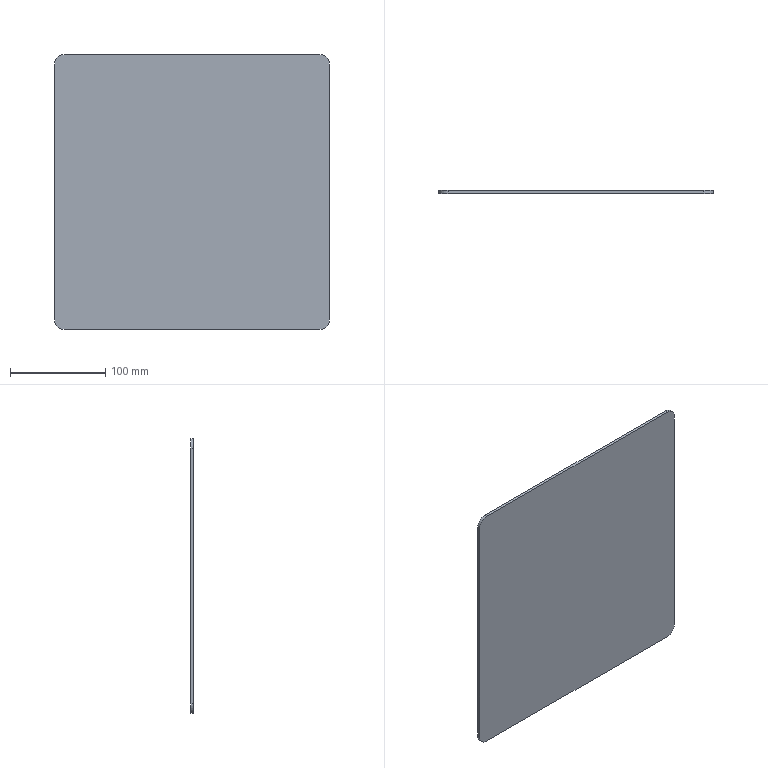Part | SolidWorks | features Extrusion 1 | 1 solid | 10 faces | box 288 x 3 x 288 mm | volume 248574 mm3 | plane 6 | cylinder 4 | commonest cylinder face diameters 20 x4
STEP:
#1=CARTESIAN_POINT('',(-144.,0.,134.));
#2=VERTEX_POINT('',#1);
#3=CARTESIAN_POINT('',(-134.,0.,144.));
#4=VERTEX_POINT('',#3);
#5=CARTESIAN_POINT('',(-134.,0.,134.));
#6=DIRECTION('',(0.,1.,0.));
#7=DIRECTION('',(0.,0.,-1.));
#8=AXIS2_PLACEMENT_3D('',#5,#6,#7);
#9=CIRCLE('',#8,10.);
#10=EDGE_CURVE('',#2,#4,#9,.T.);
#11=ORIENTED_EDGE('',*,*,#10,.T.);
#12=CARTESIAN_POINT('',(-134.,3.,144.));
#13=VERTEX_POINT('',#12);
#14=CARTESIAN_POINT('',(-134.,3.,144.));
#15=DIRECTION('',(0.,-1.,0.));
#16=VECTOR('',#15,1000.);
#17=LINE('',#14,#16);
#18=EDGE_CURVE('',#13,#4,#17,.T.);
#19=ORIENTED_EDGE('',*,*,#18,.F.);
#20=CARTESIAN_POINT('',(-144.,3.,134.));
#21=VERTEX_POINT('',#20);
#22=CARTESIAN_POINT('',(-134.,3.,134.));
#23=DIRECTION('',(0.,1.,0.));
#24=DIRECTION('',(0.,0.,-1.));
#25=AXIS2_PLACEMENT_3D('',#22,#23,#24);
#26=CIRCLE('',#25,10.);
#27=EDGE_CURVE('',#21,#13,#26,.T.);
#28=ORIENTED_EDGE('',*,*,#27,.F.);
#29=CARTESIAN_POINT('',(-144.,3.,134.));
#30=DIRECTION('',(0.,-1.,0.));
#31=VECTOR('',#30,1000.);
#32=LINE('',#29,#31);
#33=EDGE_CURVE('',#21,#2,#32,.T.);
#34=ORIENTED_EDGE('',*,*,#33,.T.);
#35=EDGE_LOOP('',(#11,#19,#28,#34));
#36=FACE_OUTER_BOUND('',#35,.T.);
#37=CARTESIAN_POINT('',(-134.,3.,134.));
#38=DIRECTION('',(0.,-1.,0.));
#39=DIRECTION('',(0.,0.,-1.));
#40=AXIS2_PLACEMENT_3D('',#37,#38,#39);
#41=CYLINDRICAL_SURFACE('',#40,10.);
#42=ADVANCED_FACE('',(#36),#41,.T.);
#43=CARTESIAN_POINT('',(134.,0.,144.));
#44=VERTEX_POINT('',#43);
#45=CARTESIAN_POINT('',(-134.,0.,144.));
#46=DIRECTION('',(1.,0.,0.));
#47=VECTOR('',#46,1000.);
#48=LINE('',#45,#47);
#49=EDGE_CURVE('',#4,#44,#48,.T.);
#50=ORIENTED_EDGE('',*,*,#49,.T.);
#51=CARTESIAN_POINT('',(134.,3.,144.));
#52=VERTEX_POINT('',#51);
#53=CARTESIAN_POINT('',(134.,3.,144.));
#54=DIRECTION('',(0.,-1.,0.));
#55=VECTOR('',#54,1000.);
#56=LINE('',#53,#55);
#57=EDGE_CURVE('',#52,#44,#56,.T.);
#58=ORIENTED_EDGE('',*,*,#57,.F.);
#59=CARTESIAN_POINT('',(-134.,3.,144.));
#60=DIRECTION('',(1.,0.,0.));
#61=VECTOR('',#60,1000.);
#62=LINE('',#59,#61);
#63=EDGE_CURVE('',#13,#52,#62,.T.);
#64=ORIENTED_EDGE('',*,*,#63,.F.);
#65=ORIENTED_EDGE('',*,*,#18,.T.);
#66=EDGE_LOOP('',(#50,#58,#64,#65));
#67=FACE_OUTER_BOUND('',#66,.T.);
#68=CARTESIAN_POINT('',(-134.,3.,144.));
#69=DIRECTION('',(0.,0.,-1.));
#70=DIRECTION('',(-1.,0.,0.));
#71=AXIS2_PLACEMENT_3D('',#68,#69,#70);
#72=PLANE('',#71);
#73=ADVANCED_FACE('',(#67),#72,.F.);
#74=CARTESIAN_POINT('',(144.,0.,134.));
#75=VERTEX_POINT('',#74);
#76=CARTESIAN_POINT('',(134.,0.,134.));
#77=DIRECTION('',(0.,1.,0.));
#78=DIRECTION('',(0.,0.,1.));
#79=AXIS2_PLACEMENT_3D('',#76,#77,#78);
#80=CIRCLE('',#79,10.);
#81=EDGE_CURVE('',#44,#75,#80,.T.);
#82=ORIENTED_EDGE('',*,*,#81,.T.);
#83=CARTESIAN_POINT('',(144.,3.,134.));
#84=VERTEX_POINT('',#83);
#85=CARTESIAN_POINT('',(144.,3.,134.));
#86=DIRECTION('',(0.,-1.,0.));
#87=VECTOR('',#86,1000.);
#88=LINE('',#85,#87);
#89=EDGE_CURVE('',#84,#75,#88,.T.);
#90=ORIENTED_EDGE('',*,*,#89,.F.);
#91=CARTESIAN_POINT('',(134.,3.,134.));
#92=DIRECTION('',(0.,1.,0.));
#93=DIRECTION('',(0.,0.,1.));
#94=AXIS2_PLACEMENT_3D('',#91,#92,#93);
#95=CIRCLE('',#94,10.);
#96=EDGE_CURVE('',#52,#84,#95,.T.);
#97=ORIENTED_EDGE('',*,*,#96,.F.);
#98=ORIENTED_EDGE('',*,*,#57,.T.);
#99=EDGE_LOOP('',(#82,#90,#97,#98));
#100=FACE_OUTER_BOUND('',#99,.T.);
#101=CARTESIAN_POINT('',(134.,3.,134.));
#102=DIRECTION('',(0.,-1.,0.));
#103=DIRECTION('',(0.,0.,-1.));
#104=AXIS2_PLACEMENT_3D('',#101,#102,#103);
#105=CYLINDRICAL_SURFACE('',#104,10.);
#106=ADVANCED_FACE('',(#100),#105,.T.);
#107=CARTESIAN_POINT('',(144.,0.,-134.));
#108=VERTEX_POINT('',#107);
#109=CARTESIAN_POINT('',(144.,0.,134.));
#110=DIRECTION('',(0.,0.,-1.));
#111=VECTOR('',#110,1000.);
#112=LINE('',#109,#111);
#113=EDGE_CURVE('',#75,#108,#112,.T.);
#114=ORIENTED_EDGE('',*,*,#113,.T.);
#115=CARTESIAN_POINT('',(144.,3.,-134.));
#116=VERTEX_POINT('',#115);
#117=CARTESIAN_POINT('',(144.,3.,-134.));
#118=DIRECTION('',(0.,-1.,0.));
#119=VECTOR('',#118,1000.);
#120=LINE('',#117,#119);
#121=EDGE_CURVE('',#116,#108,#120,.T.);
#122=ORIENTED_EDGE('',*,*,#121,.F.);
#123=CARTESIAN_POINT('',(144.,3.,134.));
#124=DIRECTION('',(0.,0.,-1.));
#125=VECTOR('',#124,1000.);
#126=LINE('',#123,#125);
#127=EDGE_CURVE('',#84,#116,#126,.T.);
#128=ORIENTED_EDGE('',*,*,#127,.F.);
#129=ORIENTED_EDGE('',*,*,#89,.T.);
#130=EDGE_LOOP('',(#114,#122,#128,#129));
#131=FACE_OUTER_BOUND('',#130,.T.);
#132=CARTESIAN_POINT('',(144.,3.,134.));
#133=DIRECTION('',(-1.,0.,0.));
#134=DIRECTION('',(0.,0.,1.));
#135=AXIS2_PLACEMENT_3D('',#132,#133,#134);
#136=PLANE('',#135);
#137=ADVANCED_FACE('',(#131),#136,.F.);
#138=CARTESIAN_POINT('',(134.,0.,-144.));
#139=VERTEX_POINT('',#138);
#140=CARTESIAN_POINT('',(134.,0.,-134.));
#141=DIRECTION('',(0.,1.,0.));
#142=DIRECTION('',(0.,0.,-1.));
#143=AXIS2_PLACEMENT_3D('',#140,#141,#142);
#144=CIRCLE('',#143,10.);
#145=EDGE_CURVE('',#108,#139,#144,.T.);
#146=ORIENTED_EDGE('',*,*,#145,.T.);
#147=CARTESIAN_POINT('',(134.,3.,-144.));
#148=VERTEX_POINT('',#147);
#149=CARTESIAN_POINT('',(134.,3.,-144.));
#150=DIRECTION('',(0.,-1.,0.));
#151=VECTOR('',#150,1000.);
#152=LINE('',#149,#151);
#153=EDGE_CURVE('',#148,#139,#152,.T.);
#154=ORIENTED_EDGE('',*,*,#153,.F.);
#155=CARTESIAN_POINT('',(134.,3.,-134.));
#156=DIRECTION('',(0.,1.,0.));
#157=DIRECTION('',(0.,0.,-1.));
#158=AXIS2_PLACEMENT_3D('',#155,#156,#157);
#159=CIRCLE('',#158,10.);
#160=EDGE_CURVE('',#116,#148,#159,.T.);
#161=ORIENTED_EDGE('',*,*,#160,.F.);
#162=ORIENTED_EDGE('',*,*,#121,.T.);
#163=EDGE_LOOP('',(#146,#154,#161,#162));
#164=FACE_OUTER_BOUND('',#163,.T.);
#165=CARTESIAN_POINT('',(134.,3.,-134.));
#166=DIRECTION('',(0.,-1.,0.));
#167=DIRECTION('',(0.,0.,-1.));
#168=AXIS2_PLACEMENT_3D('',#165,#166,#167);
#169=CYLINDRICAL_SURFACE('',#168,10.);
#170=ADVANCED_FACE('',(#164),#169,.T.);
#171=CARTESIAN_POINT('',(-134.,0.,-144.));
#172=VERTEX_POINT('',#171);
#173=CARTESIAN_POINT('',(-134.,0.,-144.));
#174=DIRECTION('',(-1.,0.,0.));
#175=VECTOR('',#174,1000.);
#176=LINE('',#173,#175);
#177=EDGE_CURVE('',#139,#172,#176,.T.);
#178=ORIENTED_EDGE('',*,*,#177,.T.);
#179=CARTESIAN_POINT('',(-134.,3.,-144.));
#180=VERTEX_POINT('',#179);
#181=CARTESIAN_POINT('',(-134.,3.,-144.));
#182=DIRECTION('',(0.,-1.,0.));
#183=VECTOR('',#182,1000.);
#184=LINE('',#181,#183);
#185=EDGE_CURVE('',#180,#172,#184,.T.);
#186=ORIENTED_EDGE('',*,*,#185,.F.);
#187=CARTESIAN_POINT('',(-134.,3.,-144.));
#188=DIRECTION('',(-1.,0.,0.));
#189=VECTOR('',#188,1000.);
#190=LINE('',#187,#189);
#191=EDGE_CURVE('',#148,#180,#190,.T.);
#192=ORIENTED_EDGE('',*,*,#191,.F.);
#193=ORIENTED_EDGE('',*,*,#153,.T.);
#194=EDGE_LOOP('',(#178,#186,#192,#193));
#195=FACE_OUTER_BOUND('',#194,.T.);
#196=CARTESIAN_POINT('',(-134.,3.,-144.));
#197=DIRECTION('',(0.,0.,1.));
#198=DIRECTION('',(1.,0.,0.));
#199=AXIS2_PLACEMENT_3D('',#196,#197,#198);
#200=PLANE('',#199);
#201=ADVANCED_FACE('',(#195),#200,.F.);
#202=CARTESIAN_POINT('',(-144.,0.,-134.));
#203=VERTEX_POINT('',#202);
#204=CARTESIAN_POINT('',(-134.,0.,-134.));
#205=DIRECTION('',(0.,1.,0.));
#206=DIRECTION('',(0.,0.,-1.));
#207=AXIS2_PLACEMENT_3D('',#204,#205,#206);
#208=CIRCLE('',#207,10.);
#209=EDGE_CURVE('',#172,#203,#208,.T.);
#210=ORIENTED_EDGE('',*,*,#209,.T.);
#211=CARTESIAN_POINT('',(-144.,3.,-134.));
#212=VERTEX_POINT('',#211);
#213=CARTESIAN_POINT('',(-144.,3.,-134.));
#214=DIRECTION('',(0.,-1.,0.));
#215=VECTOR('',#214,1000.);
#216=LINE('',#213,#215);
#217=EDGE_CURVE('',#212,#203,#216,.T.);
#218=ORIENTED_EDGE('',*,*,#217,.F.);
#219=CARTESIAN_POINT('',(-134.,3.,-134.));
#220=DIRECTION('',(0.,1.,0.));
#221=DIRECTION('',(0.,0.,-1.));
#222=AXIS2_PLACEMENT_3D('',#219,#220,#221);
#223=CIRCLE('',#222,10.);
#224=EDGE_CURVE('',#180,#212,#223,.T.);
#225=ORIENTED_EDGE('',*,*,#224,.F.);
#226=ORIENTED_EDGE('',*,*,#185,.T.);
#227=EDGE_LOOP('',(#210,#218,#225,#226));
#228=FACE_OUTER_BOUND('',#227,.T.);
#229=CARTESIAN_POINT('',(-134.,3.,-134.));
#230=DIRECTION('',(0.,-1.,0.));
#231=DIRECTION('',(0.,0.,-1.));
#232=AXIS2_PLACEMENT_3D('',#229,#230,#231);
#233=CYLINDRICAL_SURFACE('',#232,10.);
#234=ADVANCED_FACE('',(#228),#233,.T.);
#235=CARTESIAN_POINT('',(-144.,0.,134.));
#236=DIRECTION('',(0.,0.,1.));
#237=VECTOR('',#236,1000.);
#238=LINE('',#235,#237);
#239=EDGE_CURVE('',#203,#2,#238,.T.);
#240=ORIENTED_EDGE('',*,*,#239,.T.);
#241=ORIENTED_EDGE('',*,*,#33,.F.);
#242=CARTESIAN_POINT('',(-144.,3.,134.));
#243=DIRECTION('',(0.,0.,1.));
#244=VECTOR('',#243,1000.);
#245=LINE('',#242,#244);
#246=EDGE_CURVE('',#212,#21,#245,.T.);
#247=ORIENTED_EDGE('',*,*,#246,.F.);
#248=ORIENTED_EDGE('',*,*,#217,.T.);
#249=EDGE_LOOP('',(#240,#241,#247,#248));
#250=FACE_OUTER_BOUND('',#249,.T.);
#251=CARTESIAN_POINT('',(-144.,3.,134.));
#252=DIRECTION('',(1.,0.,0.));
#253=DIRECTION('',(0.,0.,-1.));
#254=AXIS2_PLACEMENT_3D('',#251,#252,#253);
#255=PLANE('',#254);
#256=ADVANCED_FACE('',(#250),#255,.F.);
#257=ORIENTED_EDGE('',*,*,#27,.T.);
#258=ORIENTED_EDGE('',*,*,#63,.T.);
#259=ORIENTED_EDGE('',*,*,#96,.T.);
#260=ORIENTED_EDGE('',*,*,#127,.T.);
#261=ORIENTED_EDGE('',*,*,#160,.T.);
#262=ORIENTED_EDGE('',*,*,#191,.T.);
#263=ORIENTED_EDGE('',*,*,#224,.T.);
#264=ORIENTED_EDGE('',*,*,#246,.T.);
#265=EDGE_LOOP('',(#257,#258,#259,#260,#261,#262,#263,#264));
#266=FACE_OUTER_BOUND('',#265,.T.);
#267=CARTESIAN_POINT('',(-134.,3.,134.));
#268=DIRECTION('',(0.,-1.,0.));
#269=DIRECTION('',(0.,0.,-1.));
#270=AXIS2_PLACEMENT_3D('',#267,#268,#269);
#271=PLANE('',#270);
#272=ADVANCED_FACE('',(#266),#271,.F.);
#273=ORIENTED_EDGE('',*,*,#10,.F.);
#274=ORIENTED_EDGE('',*,*,#239,.F.);
#275=ORIENTED_EDGE('',*,*,#209,.F.);
#276=ORIENTED_EDGE('',*,*,#177,.F.);
#277=ORIENTED_EDGE('',*,*,#145,.F.);
#278=ORIENTED_EDGE('',*,*,#113,.F.);
#279=ORIENTED_EDGE('',*,*,#81,.F.);
#280=ORIENTED_EDGE('',*,*,#49,.F.);
#281=EDGE_LOOP('',(#273,#274,#275,#276,#277,#278,#279,#280));
#282=FACE_OUTER_BOUND('',#281,.T.);
#283=CARTESIAN_POINT('',(-134.,0.,134.));
#284=DIRECTION('',(0.,-1.,0.));
#285=DIRECTION('',(0.,0.,-1.));
#286=AXIS2_PLACEMENT_3D('',#283,#284,#285);
#287=PLANE('',#286);
#288=ADVANCED_FACE('',(#282),#287,.T.);
#289=CLOSED_SHELL('',(#42,#73,#106,#137,#170,#201,#234,#256,#272,#288));
#290=MANIFOLD_SOLID_BREP('',#289);
#291=CARTESIAN_POINT('',(0.,0.,0.));
#292=DIRECTION('',(0.,0.,1.));
#293=DIRECTION('',(1.,0.,0.));
#294=AXIS2_PLACEMENT_3D('',#291,#292,#293);
#295=(LENGTH_UNIT()NAMED_UNIT(*)SI_UNIT(.MILLI.,.METRE.));
#296=UNCERTAINTY_MEASURE_WITH_UNIT(LENGTH_MEASURE(0.00001),#295,'','');
#297=(NAMED_UNIT(*)PLANE_ANGLE_UNIT()SI_UNIT($,.RADIAN.));
#298=(NAMED_UNIT(*)SI_UNIT($,.STERADIAN.)SOLID_ANGLE_UNIT());
#299=(GEOMETRIC_REPRESENTATION_CONTEXT(3)GLOBAL_UNCERTAINTY_ASSIGNED_CONTEXT((#296))GLOBAL_UNIT_ASSIGNED_CONTEXT((#295,#297,#298))REPRESENTATION_CONTEXT('',''));
#300=ADVANCED_BREP_SHAPE_REPRESENTATION('',(#290,#294),#299);